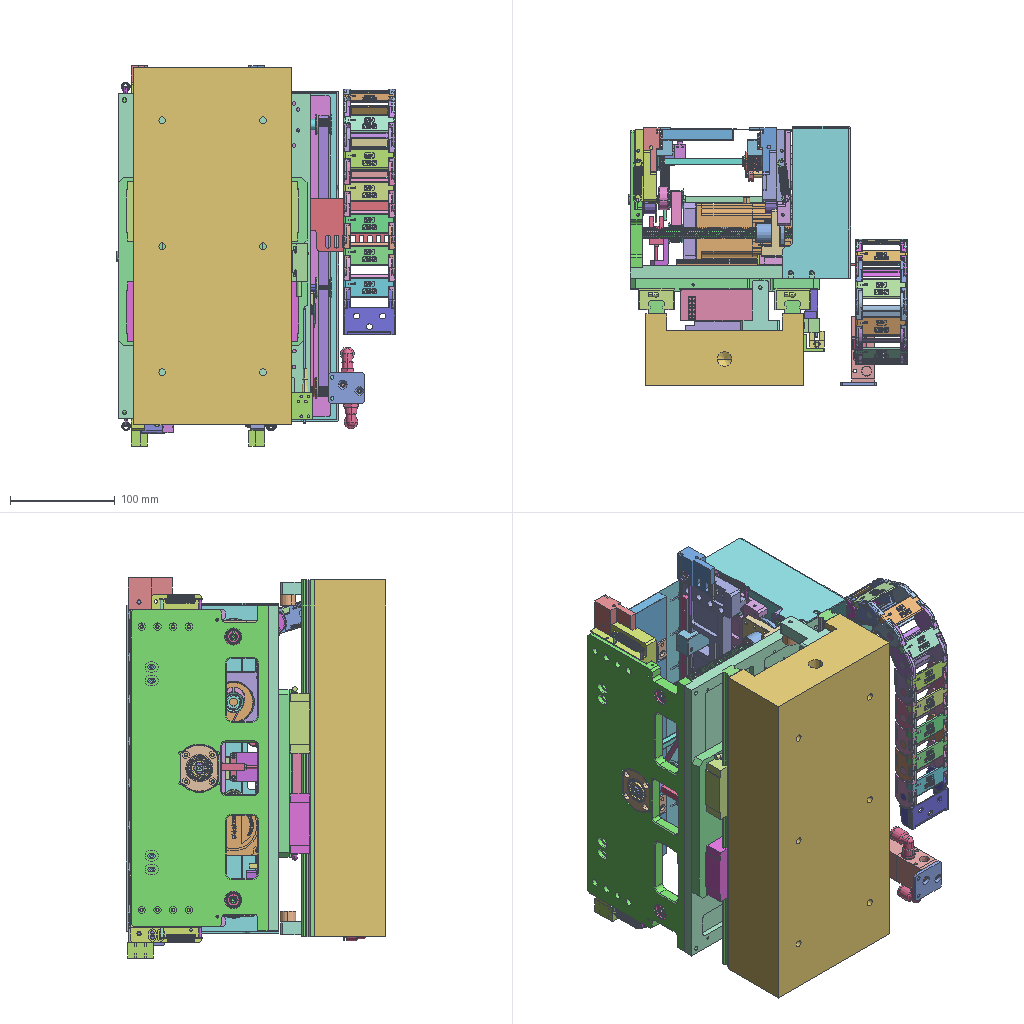Assembly | NX | 130 different items | 236 placed | box 266 x 247 x 362 mm
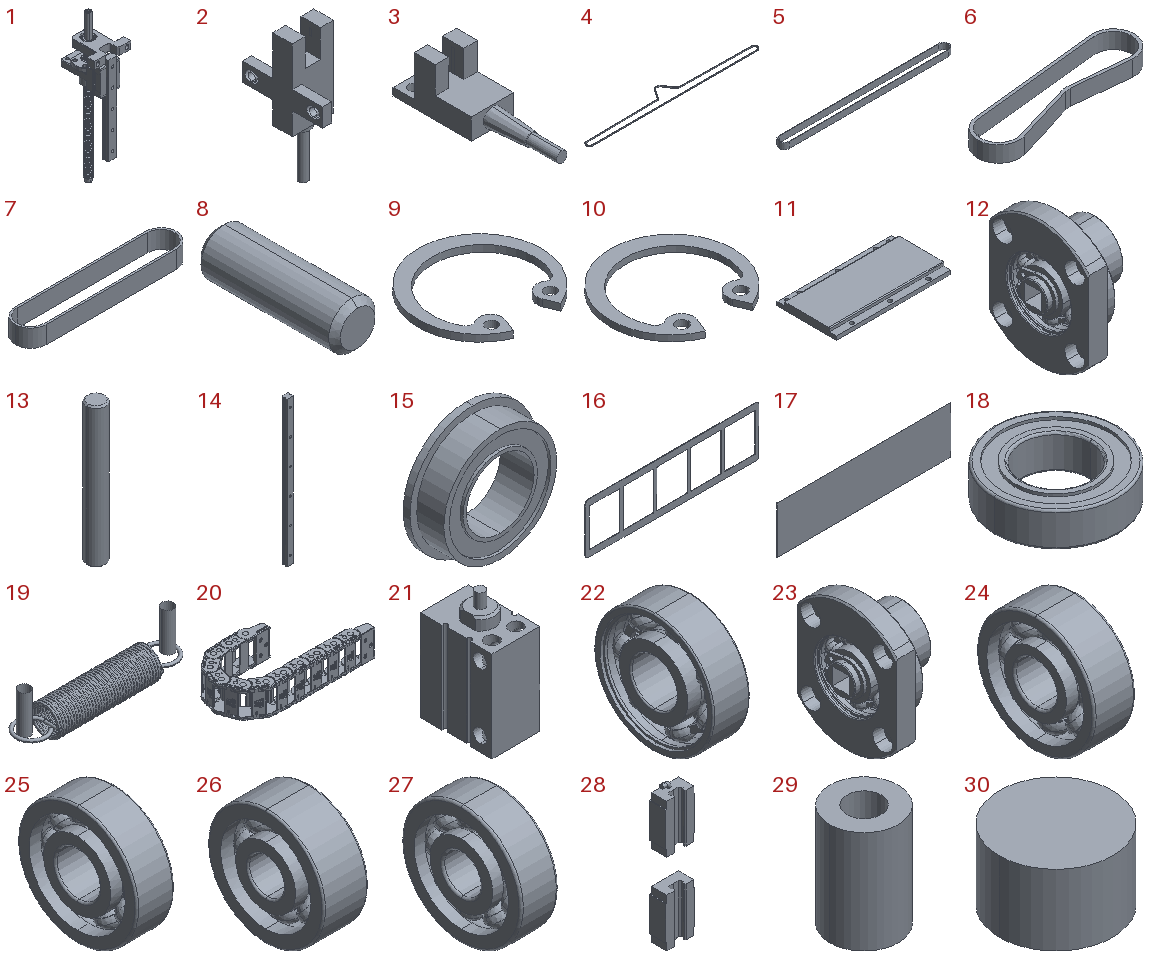Parts list (item | quantity | parent item | size | volume | features):
1 | x1 | in 42 | 50 x 56 x 201.3 mm | 60246 mm3 | features BREP 12
2 | x1 | in 42 | 13.4 x 26 x 43.2 mm | 2373 mm3 | features BREP 3
3 | x2 | in 42, 48 | 14 x 49 x 16 mm | 2990 mm3 | features BREP 1
4 | x1 | in 38 | 328.201 x 36.406 x 2 mm | 1528 mm3 | features BREP 1
5 | x1 | in 42 | 267.76 x 16.76 x 9.5 mm | 5760 mm3 | features BREP 1
6 | x1 | in 38 | 68.88 x 22.38 x 6.4 mm | 1208 mm3 | features BREP 1
7 | x2 | in 42 | 87.76 x 16.76 x 9.5 mm | 1998 mm3 | features BREP 1
8 | x2 | in 40 | 4 x 12 x 4 mm | 147.917 mm3 | features BREP 1
9 | x1 | in 46 | 18.3 x 17.603 x 1 mm | 85.781 mm3 | features BREP 1
10 | x4 | in 1, 37, 120 | 20.5 x 19.72 x 1 mm | 114.602 mm3 | features BREP 1
11 | x2 | in 48 | 143.8 x 75 x 9.2 mm | 87123 mm3 | features BREP 1
12 | x1 | in 37 | 26 x 35 x 45 mm | 12567 mm3 | features BREP 5
13 | x1 | in 45 | 4 x 4 x 30 mm | 375.917 mm3 | features BREP 1
14 | x2 | in 48 | 15 x 12.5 x 340 mm | 57238 mm3 | features BREP 1
15 | x8 | in 49, 50, 51, 52, 53, 55, 56, 57 | 11.2 x 3 x 11.2 mm | 148.082 mm3 | features BREP 1
16 | x1 | in 44 | 258 x 0.7 x 75 mm | 4535 mm3 | features BREP 1
17 | x1 | in 44 | 258 x 0.1 x 70 mm | 1806 mm3 | features BREP 1
18 | x2 | in 42 | 9 x 9 x 2.5 mm | 101.727 mm3 | features BREP 1
19 | x4 | in 40, 41 | 41.6 x 8.1 x 14 mm | 518.978 mm3 | features BREP 3
20 | x1 | in 48 | - | 130041 mm3 | features BREP 24
21 | x1 | in 45 | 10 x 15 x 24.5 mm | 2449 mm3 | features BREP 2
22 | x4 | in 12, 23, 34, 38 | 8 x 26 x 26 mm | 2122 mm3 | features BREP 1
23 | x1 | in 39 | 26 x 35 x 45 mm | 12567 mm3 | features BREP 5
24 | x1 | in 46 | 6 x 17 x 17 mm | 795.711 mm3 | features BREP 1
25 | x4 | in 1, 37, 120 | 6 x 19 x 19 mm | 1040 mm3 | features BREP 1
26 | x1 | in 38 | 5 x 13 x 13 mm | 428.524 mm3 | features BREP 1
27 | x1 | in 42 | 5 x 16 x 16 mm | 656.874 mm3 | features BREP 1
28 | x2 | in 48 | 34 x 19.5 x 165.7 mm | 60409 mm3 | features BREP 2
29 | x1 | in 45 | 8 x 8 x 12 mm | 452.389 mm3 | features BREP 1
30 | x4 | in 37, 39 | 8 x 8 x 5 mm | 251.327 mm3 | features BREP 1
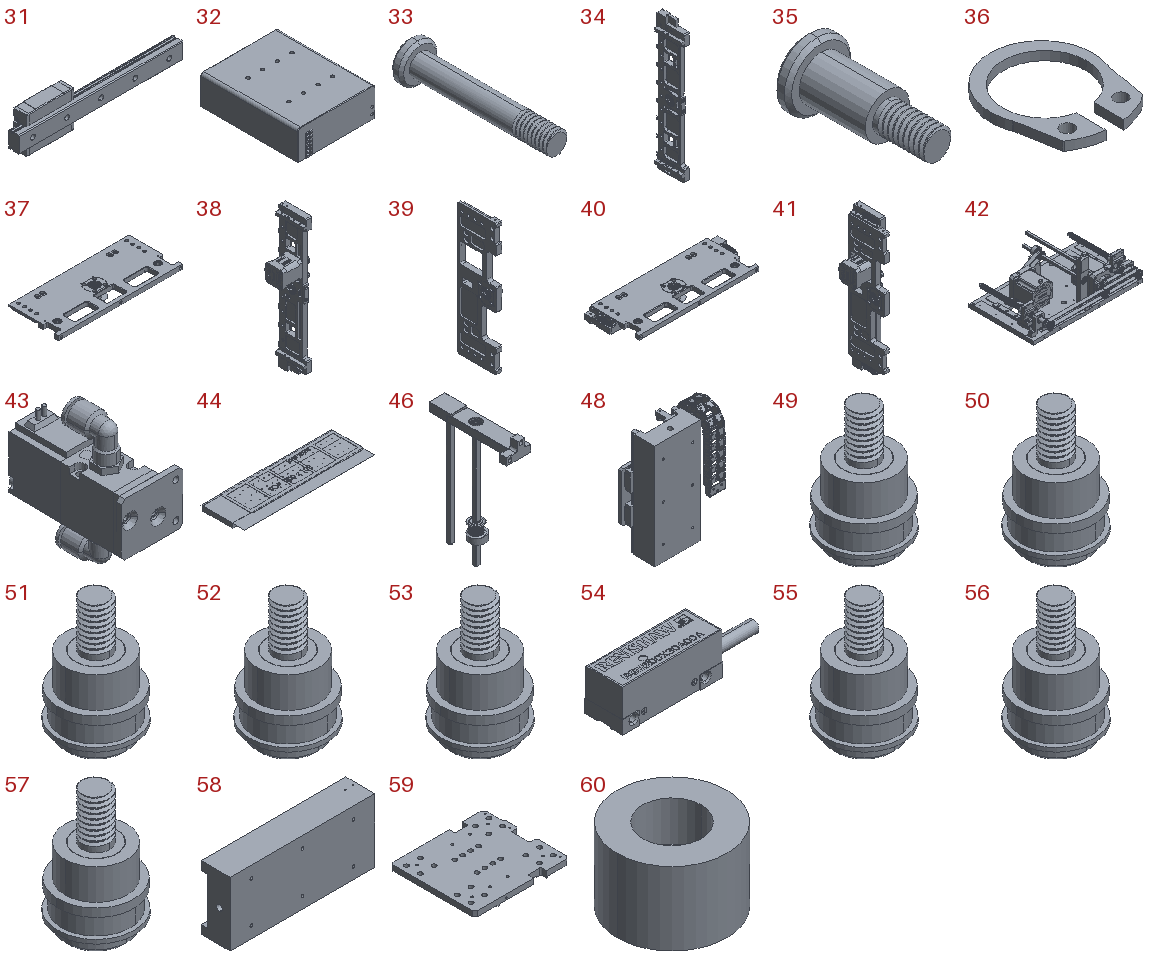31 | x2 | in 1, 120 | 120 x 13 x 27 mm | 16651 mm3 | features BREP 4
32 | x1 | in 48 | 80 x 101 x 30 mm | 238985 mm3 | features BREP 7
33 | x1 | in 38 | 7 x 27 x 7 mm | 340.818 mm3 | features BREP 1
34 | x1 | in 40 | 33.5 x 70 x 347.5 mm | 189578 mm3 | features BREP 15
35 | x8 | in 49, 50, 51, 52, 53, 55, 56, 57 | 9 x 18 x 9 mm | 417.74 mm3 | features BREP 1
36 | x6 | in 12, 23, 34, 38 | 11.5 x 13.997 x 1 mm | 53.264 mm3 | features BREP 1
37 | x1 | in 40 | 310 x 130.5 x 42 mm | 276547 mm3 | features BREP 13
38 | x1 | in 41 | - | 279184 mm3 | features BREP 23
39 | x1 | in 41 | 43 x 90 x 302 mm | 186780 mm3 | features BREP 10
40 | x1 | in 47 | - | 467322 mm3 | features BREP 29
41 | x1 | in 47 | - | 466877 mm3 | features BREP 33
42 | x1 | in 47 | - | 1088437 mm3 | features BREP 40
43 | x1 | - | 35 x 66 x 78.15 mm | 39184 mm3 | features BREP 2
44 | x1 | in 47 | 300 x 100 x 10.8 mm | 198178 mm3 | features BREP 19
45 | x1 | in 47 | - | - | features BREP 7
46 | x1 | in 42 | 37.325 x 120 x 185 mm | 44001 mm3 | features BREP 8
47 | x1 | - | - | - | features BREP 109
48 | x1 | - | - | 3906926 mm3 | features BREP 46
49 | x1 | in 34 | 11.2 x 11.2 x 18 mm | 807.329 mm3 | features BREP 4
50 | x1 | in 34 | 11.2 x 11.2 x 18 mm | 807.329 mm3 | features BREP 4
51 | x1 | in 38 | 11.2 x 11.2 x 18 mm | 807.329 mm3 | features BREP 4
52 | x1 | in 38 | 11.2 x 11.2 x 18 mm | 807.329 mm3 | features BREP 4
53 | x1 | in 38 | 11.2 x 11.2 x 18 mm | 807.329 mm3 | features BREP 4
54 | x1 | in 65 | 50.65 x 13.5 x 14.8 mm | 6947 mm3 | features BREP 1
55 | x1 | in 38 | 11.2 x 11.2 x 18 mm | 807.329 mm3 | features BREP 4
56 | x1 | in 34 | 11.2 x 11.2 x 18 mm | 807.329 mm3 | features BREP 4
57 | x1 | in 34 | 11.2 x 11.2 x 18 mm | 807.329 mm3 | features BREP 4
58 | x1 | in 48 | 340 x 68 x 150 mm | 2833787 mm3 | features BREP 1
59 | x1 | in 48 | 180 x 160 x 12 mm | 236462 mm3 | features BREP 1
60 | x2 | in 48 | 15 x 15 x 10 mm | 1419 mm3 | features BREP 1
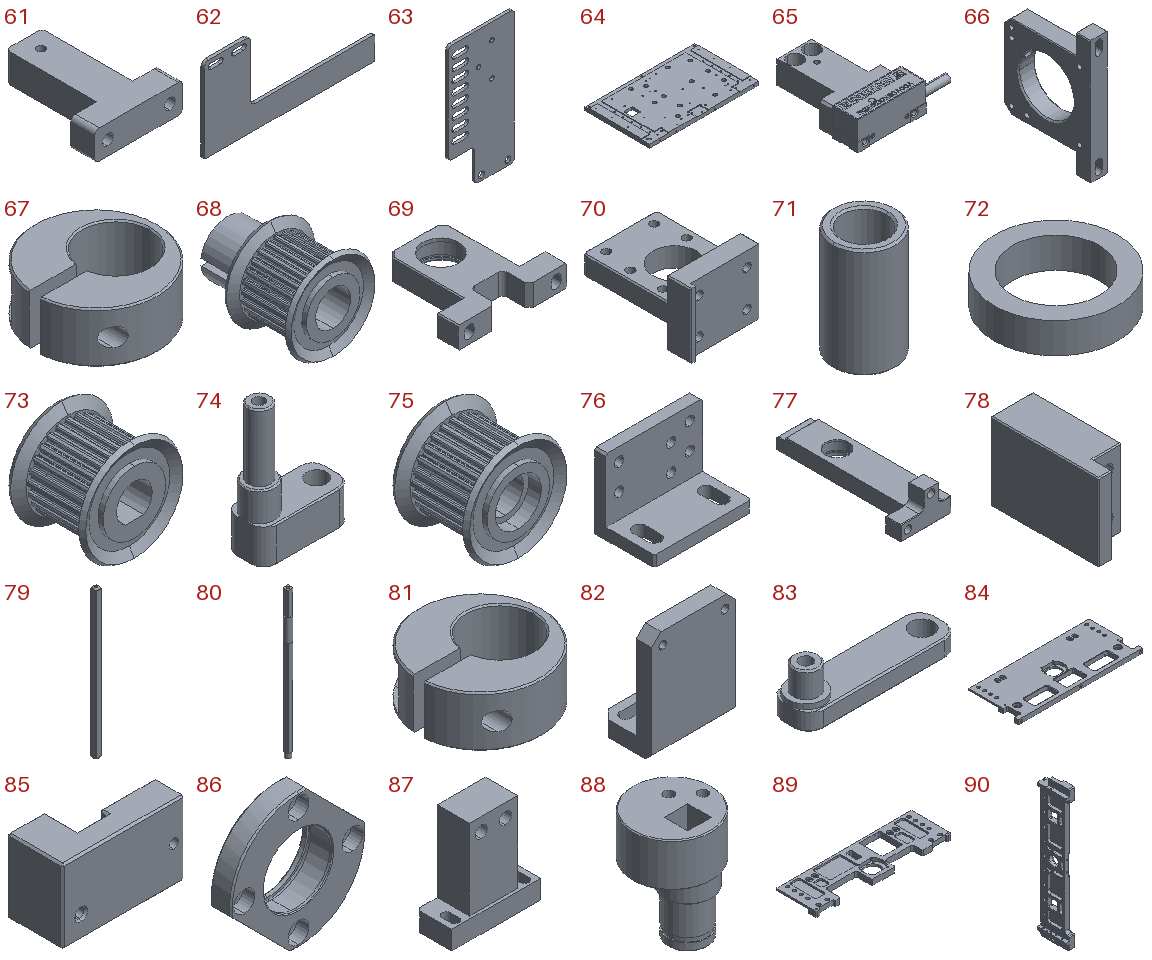61 | x2 | in 48 | 37 x 48 x 12 mm | 10327 mm3 | features BREP 1
62 | x1 | in 48 | 110 x 2 x 54 mm | 5512 mm3 | features BREP 1
63 | x1 | in 48 | 50 x 2 x 100 mm | 8039 mm3 | features BREP 1
64 | x1 | in 42 | 310 x 183.5 x 12 mm | 522912 mm3 | features BREP 1
65 | x1 | in 48 | 50.65 x 50.5 x 14.8 mm | 15333 mm3 | features BREP 2
66 | x2 | in 98, 109 | 12 x 60 x 86 mm | 28967 mm3 | features BREP 1
67 | x2 | in 98, 109 | 21.954 x 22 x 9 mm | 1945 mm3 | features BREP 1
68 | x3 | in 46, 98, 109 | 20.061 x 24 x 20.061 mm | 2586 mm3 | features BREP 1
69 | x2 | in 1, 120 | 50 x 45 x 10 mm | 8913 mm3 | features BREP 1
70 | x2 | in 1, 120 | 31 x 45 x 27 mm | 12005 mm3 | features BREP 1
71 | x1 | in 42 | 10.1 x 10.1 x 17.6 mm | 708.404 mm3 | features BREP 1
72 | x1 | in 42 | 10.1 x 10.1 x 2.5 mm | 101.316 mm3 | features BREP 1
73 | x3 | in 42 | 20.061 x 15 x 20.061 mm | 2247 mm3 | features BREP 1
74 | x1 | in 42 | 20 x 9 x 29.5 mm | 1742 mm3 | features BREP 1
75 | x1 | in 42 | 20.061 x 15 x 20.061 mm | 2125 mm3 | features BREP 1
76 | x1 | in 48 | 26 x 16 x 20 mm | 2342 mm3 | features BREP 1
77 | x1 | in 46 | 34 x 95 x 22 mm | 20298 mm3 | features BREP 1
78 | x1 | in 46 | 12 x 30.5 x 22 mm | 6571 mm3 | features BREP 1
79 | x1 | in 46 | 6 x 6 x 155 mm | 5484 mm3 | features BREP 1
80 | x1 | in 46 | 8 x 8 x 172 mm | 6270 mm3 | features BREP 1
81 | x1 | in 46 | 21.954 x 22 x 9 mm | 1911 mm3 | features BREP 1
82 | x1 | in 42 | 27 x 17 x 35 mm | 5811 mm3 | features BREP 1
83 | x1 | in 42 | 30 x 8 x 9.4 mm | 839.286 mm3 | features BREP 1
84 | x1 | in 37 | 310 x 130.5 x 11 mm | 241752 mm3 | features BREP 1
85 | x4 | in 37, 39 | 33 x 15 x 20 mm | 5682 mm3 | features BREP 1
86 | x2 | in 12, 23 | 45 x 12 x 45 mm | 6444 mm3 | features BREP 1
87 | x1 | in 65 | 33 x 13 x 37 mm | 8386 mm3 | features BREP 1
88 | x2 | in 12, 23 | 20 x 20 x 26 mm | 3745 mm3 | features BREP 1
89 | x1 | in 39 | 302 x 90 x 12 mm | 154751 mm3 | features BREP 1
90 | x1 | in 34 | 20.5 x 68 x 332 mm | 153235 mm3 | features BREP 1
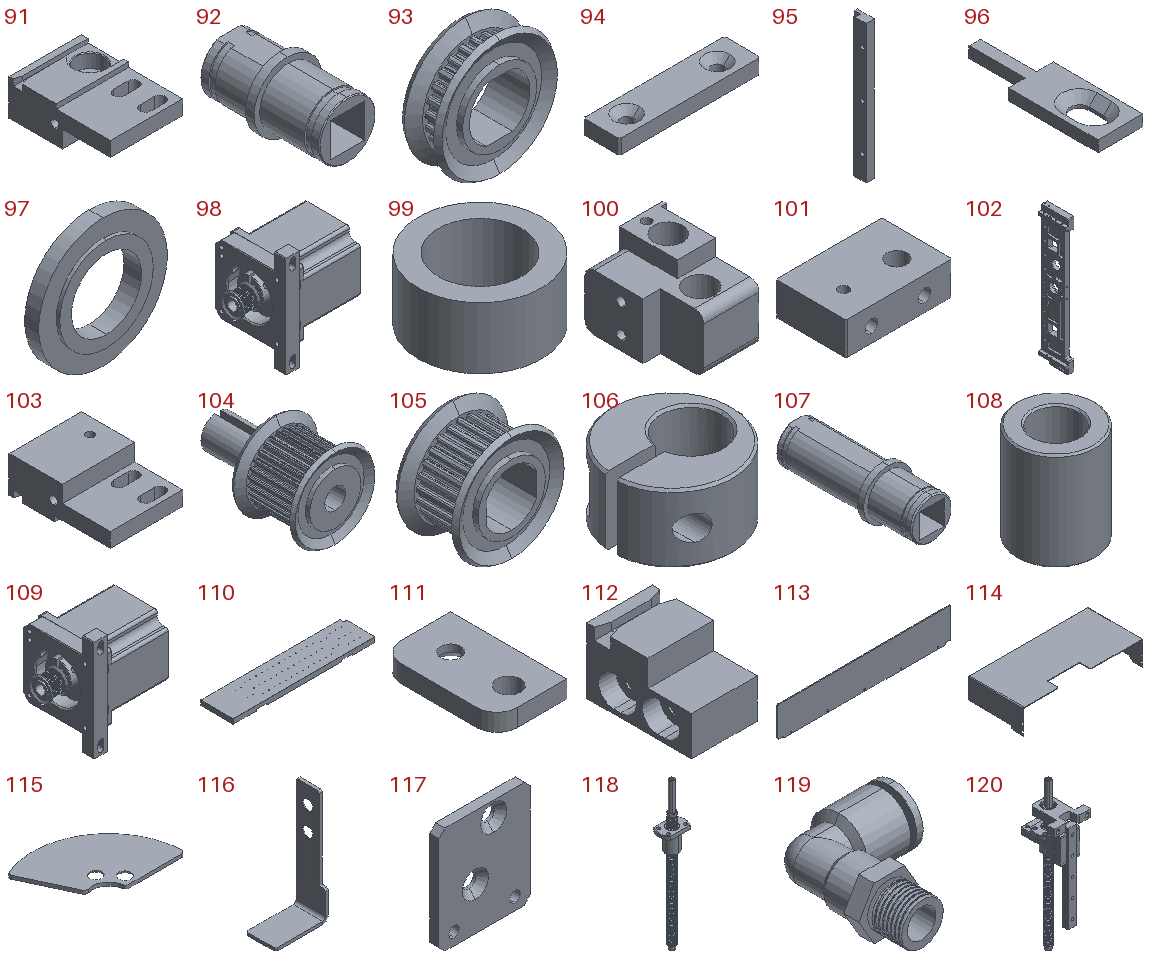91 | x1 | in 34 | 30 x 42 x 15 mm | 11527 mm3 | features BREP 1
92 | x1 | in 34 | 12 x 21 x 12 mm | 902.734 mm3 | features BREP 1
93 | x2 | in 34, 38 | 20.061 x 6.5 x 20.061 mm | 821.799 mm3 | features BREP 1
94 | x2 | in 34, 38 | 39 x 10 x 4 mm | 1439 mm3 | features BREP 1
95 | x6 | in 34, 38 | 5.3 x 11 x 89.8 mm | 4191 mm3 | features BREP 1
96 | x16 | in 34, 38 | 8 x 26 x 2 mm | 240.274 mm3 | features BREP 1
97 | x8 | in 49, 50, 51, 52, 53, 55, 56, 57 | 11 x 1.5 x 11 mm | 86.708 mm3 | features BREP 1
98 | x1 | in 42 | 80.7 x 65.2 x 86 mm | 191758 mm3 | features BREP 4
99 | x8 | in 49, 50, 51, 52, 53, 55, 56, 57 | 9 x 9 x 4.5 mm | 154.767 mm3 | features BREP 1
100 | x1 | in 45 | 21.5 x 28 x 20 mm | 6689 mm3 | features BREP 1
101 | x1 | in 45 | 21 x 14 x 6.5 mm | 1757 mm3 | features BREP 1
102 | x1 | in 38 | 20.5 x 68 x 332 mm | 151734 mm3 | features BREP 1
103 | x1 | in 38 | 30 x 42 x 15 mm | 11628 mm3 | features BREP 1
104 | x1 | in 38 | 20.061 x 28 x 20.061 mm | 2842 mm3 | features BREP 1
105 | x1 | in 38 | 20.061 x 11.5 x 20.061 mm | 1335 mm3 | features BREP 1
106 | x1 | in 38 | 15.965 x 16.002 x 9 mm | 1023 mm3 | features BREP 1
107 | x1 | in 38 | 12 x 33 x 12 mm | 1377 mm3 | features BREP 1
108 | x1 | in 38 | 7 x 7 x 8.75 mm | 220.433 mm3 | features BREP 1
109 | x1 | in 42 | 80.7 x 65.2 x 86 mm | 191758 mm3 | features BREP 4
110 | x1 | in 44 | 300 x 69 x 10 mm | 185896 mm3 | features BREP 1
111 | x4 | in 44 | 12 x 20 x 3 mm | 615.879 mm3 | features BREP 1
112 | x2 | in 47 | 15 x 24 x 15 mm | 3436 mm3 | features BREP 1
113 | x1 | in 47 | 306 x 1.5 x 56 mm | 25546 mm3 | features BREP 1
114 | x1 | in 47 | 315 x 145 x 65 mm | 112650 mm3 | features BREP 1
115 | x1 | in 37 | 31.647 x 22.5 x 1 mm | 455.867 mm3 | features BREP 1
116 | x1 | in 42 | 18 x 10 x 38 mm | 456.003 mm3 | features BREP 1
117 | x1 | in 43 | 30 x 3 x 35 mm | 2899 mm3 | features BREP 1
118 | x2 | in 1, 120 | 35 x 22 x 201.3 mm | 16501 mm3 | features BREP 4
119 | x2 | in 43 | - | - | features BREP 1
120 | x1 | in 42 | 50 x 56 x 201.3 mm | 60246 mm3 | features BREP 12
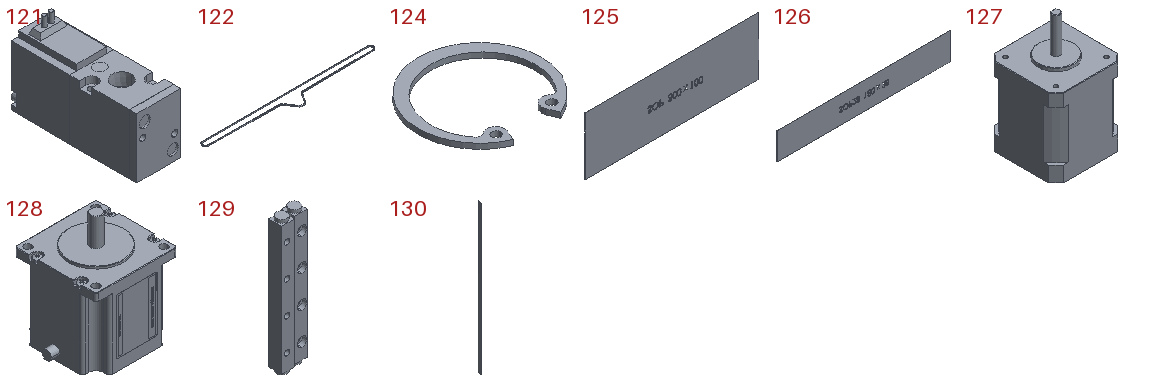121 | x1 | in 43 | 22 x 63 x 40.51 mm | 40637 mm3 | features BREP 1
122 | x1 | in 34 | 328.22 x 36.55 x 2 mm | 1530 mm3 | features BREP 1
123 | x1 | in 45 | - | - | features BREP 1
124 | x4 | in 12, 23, 34, 38 | 27.9 x 26.838 x 1.2 mm | 202.858 mm3 | features BREP 1
125 | x1 | in 44 | 300 x 0.1 x 100 mm | 2979 mm3 | features BREP 7
126 | x1 | in 44 | 180 x 0.1 x 28 mm | 498.027 mm3 | features BREP 8
127 | x1 | in 38 | 47.3 x 42.4 x 72.2 mm | 83104 mm3 | features BREP 1
128 | x2 | in 98, 109 | 62.4 x 56.5 x 75.2 mm | 158259 mm3 | features BREP 1
129 | x4 | in 37, 39 | 12 x 6 x 64 mm | 3797 mm3 | features BREP 2
130 | x1 | in 48 | 0.3 x 6 x 240 mm | 432 mm3 | features BREP 1